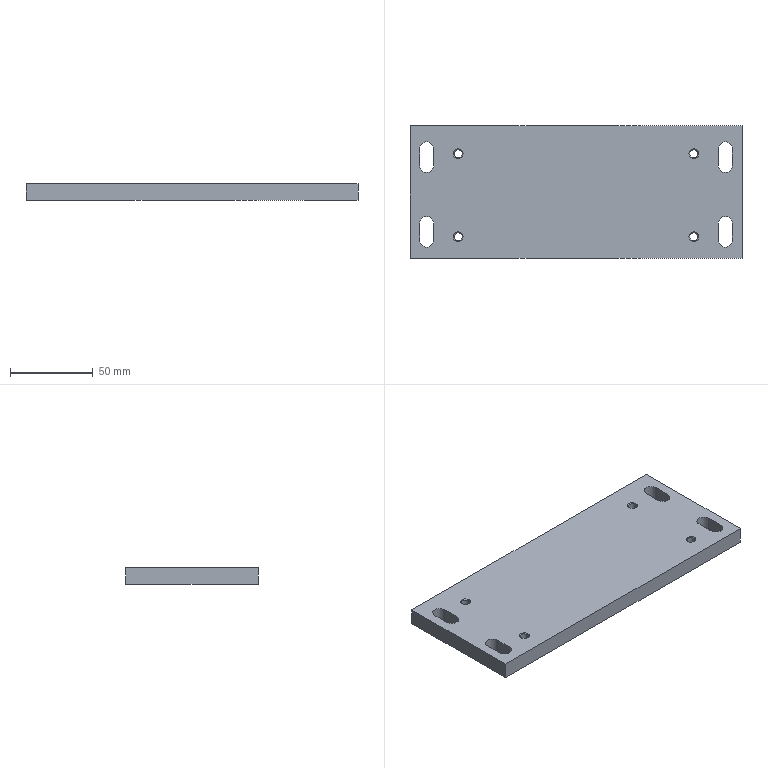Part | STEP file | Feed motor plate | 1 solid | 46 faces | box 200 x 80 x 10 mm | volume 153554 mm3 | cone 16 | cylinder 16 | plane 14 | commonest cylinder face diameters 4.917 x8 8.5 x8